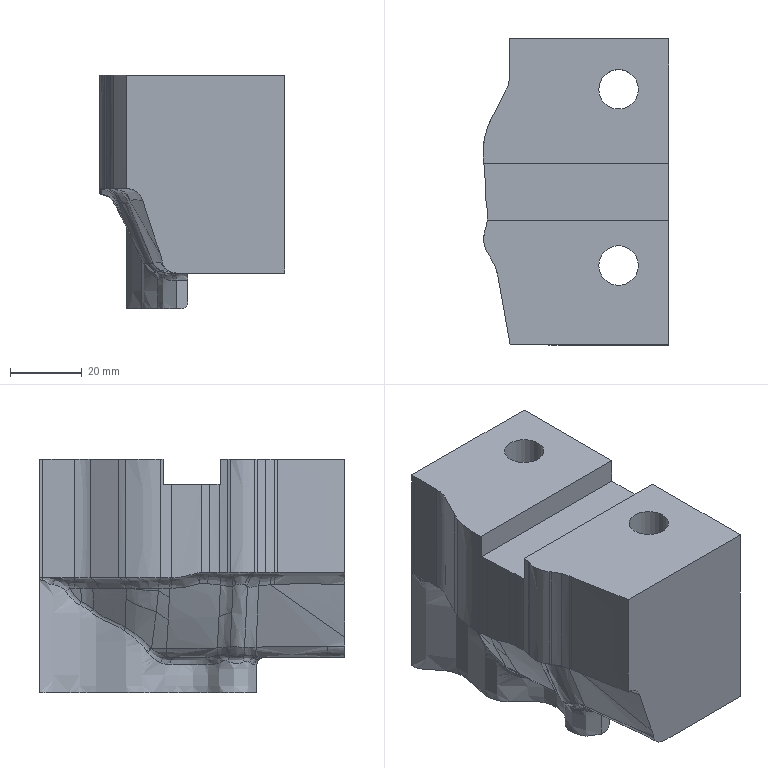Part | STEP file | PN_0030_id186_x_t | 1 solid | 106 faces | box 51.676 x 85 x 65 mm | volume 145641 mm3 | spline 64 | plane 20 | other 13 | cylinder 8 | sphere 1 | commonest cylinder face diameters 10 x3 11 x2 17 x2 4 x1